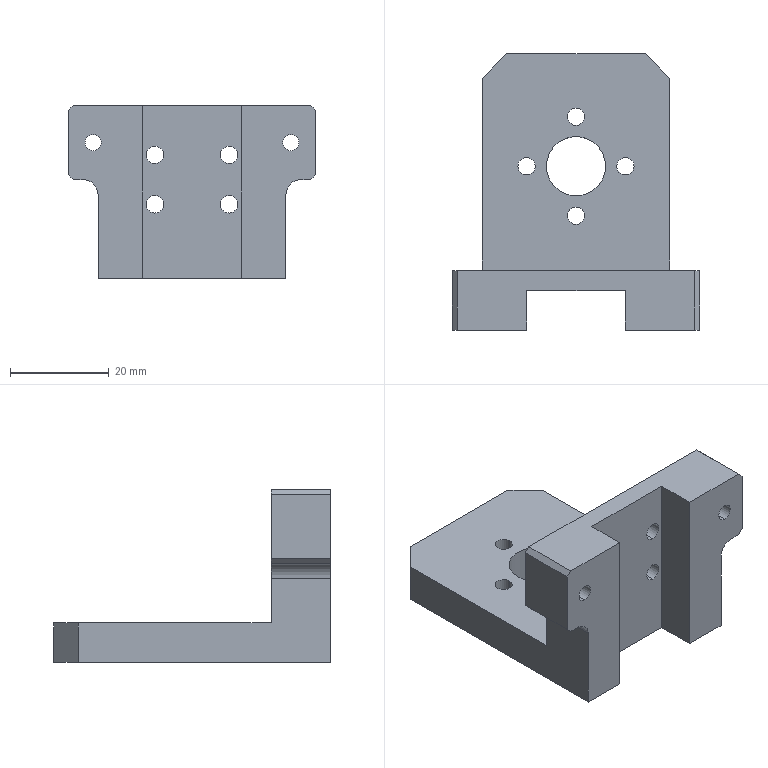Part | SolidWorks | features ICE 6, Chamfer 2, HoleWzd 2, Extrusion 1, Fillet 1 | 1 solid | 50 faces | box 50 x 56 x 35 mm | volume 24108 mm3 | cylinder 26 | plane 22 | cone 2 | commonest cylinder face diameters 3.5 x16 3.3 x4 2.5 x2 6 x2 12 x2